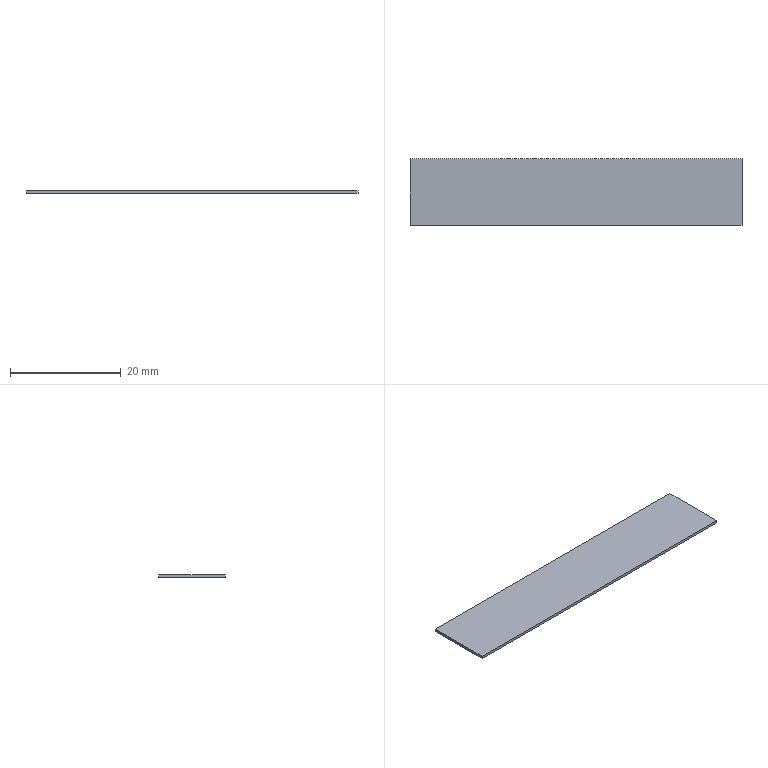Part | STEP file | 0232_013_TMEPN-2000 | 1 solid | 6 faces | box 60 x 12 x 0.5 mm | volume 359.998 mm3 | plane 6
STEP:
#1=CARTESIAN_POINT('',(0.,0.,0.));
#2=DIRECTION('',(0.,0.,1.));
#3=DIRECTION('',(1.,0.,0.));
#4=AXIS2_PLACEMENT_3D('',#1,#2,#3);
#5=CARTESIAN_POINT('',(0.,0.,0.));
#6=VERTEX_POINT('',#5);
#7=CARTESIAN_POINT('',(60.,0.,0.));
#8=VERTEX_POINT('',#7);
#9=CARTESIAN_POINT('',(60.,0.,0.));
#10=DIRECTION('',(1.,0.,0.));
#11=VECTOR('',#10,1.);
#12=LINE('',#9,#11);
#13=CARTESIAN_POINT('',(60.,6.,0.));
#14=DIRECTION('',(0.,0.,1.));
#15=DIRECTION('',(1.,0.,0.));
#16=AXIS2_PLACEMENT_3D('',#13,#14,#15);
#17=PLANE('',#16);
#18=CARTESIAN_POINT('',(0.,-6.));
#19=DIRECTION('',(1.,0.));
#20=VECTOR('',#19,1.);
#21=LINE('',#18,#20);
#22=(GEOMETRIC_REPRESENTATION_CONTEXT(2)PARAMETRIC_REPRESENTATION_CONTEXT()REPRESENTATION_CONTEXT('',''));
#23=DEFINITIONAL_REPRESENTATION('',(#21),#22);
#24=PCURVE('',#17,#23);
#25=CARTESIAN_POINT('',(1.,0.,0.));
#26=DIRECTION('',(0.,-1.,0.));
#27=DIRECTION('',(0.,0.,-1.));
#28=AXIS2_PLACEMENT_3D('',#25,#26,#27);
#29=PLANE('',#28);
#30=CARTESIAN_POINT('',(0.,59.));
#31=DIRECTION('',(0.,1.));
#32=VECTOR('',#31,1.);
#33=LINE('',#30,#32);
#34=(GEOMETRIC_REPRESENTATION_CONTEXT(2)PARAMETRIC_REPRESENTATION_CONTEXT()REPRESENTATION_CONTEXT('',''));
#35=DEFINITIONAL_REPRESENTATION('',(#33),#34);
#36=PCURVE('',#29,#35);
#37=SURFACE_CURVE('',#12,(#24,#36),.PCURVE_S1.);
#38=EDGE_CURVE('',#6,#8,#37,.T.);
#39=ORIENTED_EDGE('',*,*,#38,.F.);
#40=CARTESIAN_POINT('',(0.,12.,0.));
#41=VERTEX_POINT('',#40);
#42=CARTESIAN_POINT('',(0.,6.,0.));
#43=DIRECTION('',(0.,-1.,0.));
#44=VECTOR('',#43,1.);
#45=LINE('',#42,#44);
#46=CARTESIAN_POINT('',(-60.,0.));
#47=DIRECTION('',(0.,-1.));
#48=VECTOR('',#47,1.);
#49=LINE('',#46,#48);
#50=(GEOMETRIC_REPRESENTATION_CONTEXT(2)PARAMETRIC_REPRESENTATION_CONTEXT()REPRESENTATION_CONTEXT('',''));
#51=DEFINITIONAL_REPRESENTATION('',(#49),#50);
#52=PCURVE('',#17,#51);
#53=CARTESIAN_POINT('',(0.,0.,0.));
#54=DIRECTION('',(-1.,0.,0.));
#55=DIRECTION('',(0.,0.,1.));
#56=AXIS2_PLACEMENT_3D('',#53,#54,#55);
#57=PLANE('',#56);
#58=CARTESIAN_POINT('',(0.,6.));
#59=DIRECTION('',(0.,-1.));
#60=VECTOR('',#59,1.);
#61=LINE('',#58,#60);
#62=(GEOMETRIC_REPRESENTATION_CONTEXT(2)PARAMETRIC_REPRESENTATION_CONTEXT()REPRESENTATION_CONTEXT('',''));
#63=DEFINITIONAL_REPRESENTATION('',(#61),#62);
#64=PCURVE('',#57,#63);
#65=SURFACE_CURVE('',#45,(#52,#64),.PCURVE_S1.);
#66=EDGE_CURVE('',#41,#6,#65,.T.);
#67=ORIENTED_EDGE('',*,*,#66,.F.);
#68=CARTESIAN_POINT('',(60.,12.,0.));
#69=VERTEX_POINT('',#68);
#70=CARTESIAN_POINT('',(60.,12.,0.));
#71=DIRECTION('',(-1.,0.,0.));
#72=VECTOR('',#71,1.);
#73=LINE('',#70,#72);
#74=CARTESIAN_POINT('',(0.,6.));
#75=DIRECTION('',(-1.,0.));
#76=VECTOR('',#75,1.);
#77=LINE('',#74,#76);
#78=(GEOMETRIC_REPRESENTATION_CONTEXT(2)PARAMETRIC_REPRESENTATION_CONTEXT()REPRESENTATION_CONTEXT('',''));
#79=DEFINITIONAL_REPRESENTATION('',(#77),#78);
#80=PCURVE('',#17,#79);
#81=CARTESIAN_POINT('',(119.,12.,0.));
#82=DIRECTION('',(0.,1.,0.));
#83=DIRECTION('',(0.,0.,1.));
#84=AXIS2_PLACEMENT_3D('',#81,#82,#83);
#85=PLANE('',#84);
#86=CARTESIAN_POINT('',(0.,-59.));
#87=DIRECTION('',(0.,-1.));
#88=VECTOR('',#87,1.);
#89=LINE('',#86,#88);
#90=(GEOMETRIC_REPRESENTATION_CONTEXT(2)PARAMETRIC_REPRESENTATION_CONTEXT()REPRESENTATION_CONTEXT('',''));
#91=DEFINITIONAL_REPRESENTATION('',(#89),#90);
#92=PCURVE('',#85,#91);
#93=SURFACE_CURVE('',#73,(#80,#92),.PCURVE_S1.);
#94=EDGE_CURVE('',#69,#41,#93,.T.);
#95=ORIENTED_EDGE('',*,*,#94,.F.);
#96=CARTESIAN_POINT('',(60.,6.,0.));
#97=DIRECTION('',(0.,1.,0.));
#98=VECTOR('',#97,1.);
#99=LINE('',#96,#98);
#100=CARTESIAN_POINT('',(-0.00012,0.));
#101=DIRECTION('',(0.,1.));
#102=VECTOR('',#101,1.);
#103=LINE('',#100,#102);
#104=(GEOMETRIC_REPRESENTATION_CONTEXT(2)PARAMETRIC_REPRESENTATION_CONTEXT()REPRESENTATION_CONTEXT('',''));
#105=DEFINITIONAL_REPRESENTATION('',(#103),#104);
#106=PCURVE('',#17,#105);
#107=CARTESIAN_POINT('',(60.,12.,0.5));
#108=DIRECTION('',(-1.,0.,0.));
#109=DIRECTION('',(0.,0.,1.));
#110=AXIS2_PLACEMENT_3D('',#107,#108,#109);
#111=PLANE('',#110);
#112=CARTESIAN_POINT('',(-0.5,-6.));
#113=DIRECTION('',(0.,1.));
#114=VECTOR('',#113,1.);
#115=LINE('',#112,#114);
#116=(GEOMETRIC_REPRESENTATION_CONTEXT(2)PARAMETRIC_REPRESENTATION_CONTEXT()REPRESENTATION_CONTEXT('',''));
#117=DEFINITIONAL_REPRESENTATION('',(#115),#116);
#118=PCURVE('',#111,#117);
#119=SURFACE_CURVE('',#99,(#106,#118),.PCURVE_S1.);
#120=EDGE_CURVE('',#8,#69,#119,.T.);
#121=ORIENTED_EDGE('',*,*,#120,.F.);
#122=EDGE_LOOP('',(#39,#67,#95,#121));
#123=FACE_BOUND('',#122,.T.);
#124=ADVANCED_FACE('',(#123),#17,.F.);
#125=CARTESIAN_POINT('',(60.,12.,0.5));
#126=VERTEX_POINT('',#125);
#127=CARTESIAN_POINT('',(60.,12.,0.5));
#128=DIRECTION('',(0.,0.,-1.));
#129=VECTOR('',#128,1.);
#130=LINE('',#127,#129);
#131=CARTESIAN_POINT('',(0.,0.));
#132=DIRECTION('',(-1.,0.));
#133=VECTOR('',#132,1.);
#134=LINE('',#131,#133);
#135=(GEOMETRIC_REPRESENTATION_CONTEXT(2)PARAMETRIC_REPRESENTATION_CONTEXT()REPRESENTATION_CONTEXT('',''));
#136=DEFINITIONAL_REPRESENTATION('',(#134),#135);
#137=PCURVE('',#111,#136);
#138=CARTESIAN_POINT('',(0.5,-59.));
#139=DIRECTION('',(-1.,0.));
#140=VECTOR('',#139,1.);
#141=LINE('',#138,#140);
#142=(GEOMETRIC_REPRESENTATION_CONTEXT(2)PARAMETRIC_REPRESENTATION_CONTEXT()REPRESENTATION_CONTEXT('',''));
#143=DEFINITIONAL_REPRESENTATION('',(#141),#142);
#144=PCURVE('',#85,#143);
#145=SURFACE_CURVE('',#130,(#137,#144),.PCURVE_S1.);
#146=EDGE_CURVE('',#126,#69,#145,.T.);
#147=ORIENTED_EDGE('',*,*,#146,.F.);
#148=CARTESIAN_POINT('',(60.,0.,0.5));
#149=VERTEX_POINT('',#148);
#150=CARTESIAN_POINT('',(60.,12.,0.5));
#151=DIRECTION('',(0.,1.,0.));
#152=VECTOR('',#151,1.);
#153=LINE('',#150,#152);
#154=CARTESIAN_POINT('',(0.,0.));
#155=DIRECTION('',(0.,1.));
#156=VECTOR('',#155,1.);
#157=LINE('',#154,#156);
#158=(GEOMETRIC_REPRESENTATION_CONTEXT(2)PARAMETRIC_REPRESENTATION_CONTEXT()REPRESENTATION_CONTEXT('',''));
#159=DEFINITIONAL_REPRESENTATION('',(#157),#158);
#160=PCURVE('',#111,#159);
#161=CARTESIAN_POINT('',(60.,6.,0.5));
#162=DIRECTION('',(0.,0.,1.));
#163=DIRECTION('',(1.,0.,0.));
#164=AXIS2_PLACEMENT_3D('',#161,#162,#163);
#165=PLANE('',#164);
#166=CARTESIAN_POINT('',(-0.00012,6.));
#167=DIRECTION('',(0.,1.));
#168=VECTOR('',#167,1.);
#169=LINE('',#166,#168);
#170=(GEOMETRIC_REPRESENTATION_CONTEXT(2)PARAMETRIC_REPRESENTATION_CONTEXT()REPRESENTATION_CONTEXT('',''));
#171=DEFINITIONAL_REPRESENTATION('',(#169),#170);
#172=PCURVE('',#165,#171);
#173=SURFACE_CURVE('',#153,(#160,#172),.PCURVE_S1.);
#174=EDGE_CURVE('',#149,#126,#173,.T.);
#175=ORIENTED_EDGE('',*,*,#174,.F.);
#176=CARTESIAN_POINT('',(60.,0.,0.5));
#177=DIRECTION('',(0.,0.,1.));
#178=VECTOR('',#177,1.);
#179=LINE('',#176,#178);
#180=CARTESIAN_POINT('',(0.,-12.));
#181=DIRECTION('',(1.,0.));
#182=VECTOR('',#181,1.);
#183=LINE('',#180,#182);
#184=(GEOMETRIC_REPRESENTATION_CONTEXT(2)PARAMETRIC_REPRESENTATION_CONTEXT()REPRESENTATION_CONTEXT('',''));
#185=DEFINITIONAL_REPRESENTATION('',(#183),#184);
#186=PCURVE('',#111,#185);
#187=CARTESIAN_POINT('',(-0.5,59.));
#188=DIRECTION('',(-1.,0.));
#189=VECTOR('',#188,1.);
#190=LINE('',#187,#189);
#191=(GEOMETRIC_REPRESENTATION_CONTEXT(2)PARAMETRIC_REPRESENTATION_CONTEXT()REPRESENTATION_CONTEXT('',''));
#192=DEFINITIONAL_REPRESENTATION('',(#190),#191);
#193=PCURVE('',#29,#192);
#194=SURFACE_CURVE('',#179,(#186,#193),.PCURVE_S1.);
#195=EDGE_CURVE('',#8,#149,#194,.T.);
#196=ORIENTED_EDGE('',*,*,#195,.F.);
#197=ORIENTED_EDGE('',*,*,#120,.T.);
#198=EDGE_LOOP('',(#147,#175,#196,#197));
#199=FACE_BOUND('',#198,.T.);
#200=ADVANCED_FACE('',(#199),#111,.F.);
#201=CARTESIAN_POINT('',(0.,0.,0.5));
#202=VERTEX_POINT('',#201);
#203=CARTESIAN_POINT('',(0.,0.,0.));
#204=DIRECTION('',(0.,0.,-1.));
#205=VECTOR('',#204,1.);
#206=LINE('',#203,#205);
#207=CARTESIAN_POINT('',(0.,-1.));
#208=DIRECTION('',(1.,0.));
#209=VECTOR('',#208,1.);
#210=LINE('',#207,#209);
#211=(GEOMETRIC_REPRESENTATION_CONTEXT(2)PARAMETRIC_REPRESENTATION_CONTEXT()REPRESENTATION_CONTEXT('',''));
#212=DEFINITIONAL_REPRESENTATION('',(#210),#211);
#213=PCURVE('',#29,#212);
#214=CARTESIAN_POINT('',(0.,0.));
#215=DIRECTION('',(-1.,0.));
#216=VECTOR('',#215,1.);
#217=LINE('',#214,#216);
#218=(GEOMETRIC_REPRESENTATION_CONTEXT(2)PARAMETRIC_REPRESENTATION_CONTEXT()REPRESENTATION_CONTEXT('',''));
#219=DEFINITIONAL_REPRESENTATION('',(#217),#218);
#220=PCURVE('',#57,#219);
#221=SURFACE_CURVE('',#206,(#213,#220),.PCURVE_S1.);
#222=EDGE_CURVE('',#202,#6,#221,.T.);
#223=ORIENTED_EDGE('',*,*,#222,.T.);
#224=ORIENTED_EDGE('',*,*,#38,.T.);
#225=ORIENTED_EDGE('',*,*,#195,.T.);
#226=CARTESIAN_POINT('',(1.,0.,0.5));
#227=DIRECTION('',(-1.,0.,0.));
#228=VECTOR('',#227,1.);
#229=LINE('',#226,#228);
#230=CARTESIAN_POINT('',(-0.5,0.));
#231=DIRECTION('',(0.,-1.));
#232=VECTOR('',#231,1.);
#233=LINE('',#230,#232);
#234=(GEOMETRIC_REPRESENTATION_CONTEXT(2)PARAMETRIC_REPRESENTATION_CONTEXT()REPRESENTATION_CONTEXT('',''));
#235=DEFINITIONAL_REPRESENTATION('',(#233),#234);
#236=PCURVE('',#29,#235);
#237=CARTESIAN_POINT('',(-59.,-6.));
#238=DIRECTION('',(-1.,0.));
#239=VECTOR('',#238,1.);
#240=LINE('',#237,#239);
#241=(GEOMETRIC_REPRESENTATION_CONTEXT(2)PARAMETRIC_REPRESENTATION_CONTEXT()REPRESENTATION_CONTEXT('',''));
#242=DEFINITIONAL_REPRESENTATION('',(#240),#241);
#243=PCURVE('',#165,#242);
#244=SURFACE_CURVE('',#229,(#236,#243),.PCURVE_S1.);
#245=EDGE_CURVE('',#149,#202,#244,.T.);
#246=ORIENTED_EDGE('',*,*,#245,.T.);
#247=EDGE_LOOP('',(#223,#224,#225,#246));
#248=FACE_BOUND('',#247,.T.);
#249=ADVANCED_FACE('',(#248),#29,.T.);
#250=ORIENTED_EDGE('',*,*,#66,.T.);
#251=ORIENTED_EDGE('',*,*,#222,.F.);
#252=CARTESIAN_POINT('',(0.,12.,0.5));
#253=VERTEX_POINT('',#252);
#254=CARTESIAN_POINT('',(0.,0.,0.5));
#255=DIRECTION('',(0.,1.,0.));
#256=VECTOR('',#255,1.);
#257=LINE('',#254,#256);
#258=CARTESIAN_POINT('',(0.5,0.));
#259=DIRECTION('',(0.,1.));
#260=VECTOR('',#259,1.);
#261=LINE('',#258,#260);
#262=(GEOMETRIC_REPRESENTATION_CONTEXT(2)PARAMETRIC_REPRESENTATION_CONTEXT()REPRESENTATION_CONTEXT('',''));
#263=DEFINITIONAL_REPRESENTATION('',(#261),#262);
#264=PCURVE('',#57,#263);
#265=CARTESIAN_POINT('',(-60.,-6.));
#266=DIRECTION('',(0.,1.));
#267=VECTOR('',#266,1.);
#268=LINE('',#265,#267);
#269=(GEOMETRIC_REPRESENTATION_CONTEXT(2)PARAMETRIC_REPRESENTATION_CONTEXT()REPRESENTATION_CONTEXT('',''));
#270=DEFINITIONAL_REPRESENTATION('',(#268),#269);
#271=PCURVE('',#165,#270);
#272=SURFACE_CURVE('',#257,(#264,#271),.PCURVE_S1.);
#273=EDGE_CURVE('',#202,#253,#272,.T.);
#274=ORIENTED_EDGE('',*,*,#273,.T.);
#275=CARTESIAN_POINT('',(0.,12.,0.));
#276=DIRECTION('',(0.,0.,-1.));
#277=VECTOR('',#276,1.);
#278=LINE('',#275,#277);
#279=CARTESIAN_POINT('',(0.,12.));
#280=DIRECTION('',(-1.,0.));
#281=VECTOR('',#280,1.);
#282=LINE('',#279,#281);
#283=(GEOMETRIC_REPRESENTATION_CONTEXT(2)PARAMETRIC_REPRESENTATION_CONTEXT()REPRESENTATION_CONTEXT('',''));
#284=DEFINITIONAL_REPRESENTATION('',(#282),#283);
#285=PCURVE('',#57,#284);
#286=CARTESIAN_POINT('',(0.,-119.));
#287=DIRECTION('',(-1.,0.));
#288=VECTOR('',#287,1.);
#289=LINE('',#286,#288);
#290=(GEOMETRIC_REPRESENTATION_CONTEXT(2)PARAMETRIC_REPRESENTATION_CONTEXT()REPRESENTATION_CONTEXT('',''));
#291=DEFINITIONAL_REPRESENTATION('',(#289),#290);
#292=PCURVE('',#85,#291);
#293=SURFACE_CURVE('',#278,(#285,#292),.PCURVE_S1.);
#294=EDGE_CURVE('',#253,#41,#293,.T.);
#295=ORIENTED_EDGE('',*,*,#294,.T.);
#296=EDGE_LOOP('',(#250,#251,#274,#295));
#297=FACE_BOUND('',#296,.T.);
#298=ADVANCED_FACE('',(#297),#57,.T.);
#299=ORIENTED_EDGE('',*,*,#294,.F.);
#300=CARTESIAN_POINT('',(119.,12.,0.5));
#301=DIRECTION('',(1.,0.,0.));
#302=VECTOR('',#301,1.);
#303=LINE('',#300,#302);
#304=CARTESIAN_POINT('',(0.5,0.));
#305=DIRECTION('',(0.,1.));
#306=VECTOR('',#305,1.);
#307=LINE('',#304,#306);
#308=(GEOMETRIC_REPRESENTATION_CONTEXT(2)PARAMETRIC_REPRESENTATION_CONTEXT()REPRESENTATION_CONTEXT('',''));
#309=DEFINITIONAL_REPRESENTATION('',(#307),#308);
#310=PCURVE('',#85,#309);
#311=CARTESIAN_POINT('',(59.,6.));
#312=DIRECTION('',(1.,0.));
#313=VECTOR('',#312,1.);
#314=LINE('',#311,#313);
#315=(GEOMETRIC_REPRESENTATION_CONTEXT(2)PARAMETRIC_REPRESENTATION_CONTEXT()REPRESENTATION_CONTEXT('',''));
#316=DEFINITIONAL_REPRESENTATION('',(#314),#315);
#317=PCURVE('',#165,#316);
#318=SURFACE_CURVE('',#303,(#310,#317),.PCURVE_S1.);
#319=EDGE_CURVE('',#253,#126,#318,.T.);
#320=ORIENTED_EDGE('',*,*,#319,.T.);
#321=ORIENTED_EDGE('',*,*,#146,.T.);
#322=ORIENTED_EDGE('',*,*,#94,.T.);
#323=EDGE_LOOP('',(#299,#320,#321,#322));
#324=FACE_BOUND('',#323,.T.);
#325=ADVANCED_FACE('',(#324),#85,.T.);
#326=ORIENTED_EDGE('',*,*,#273,.F.);
#327=ORIENTED_EDGE('',*,*,#245,.F.);
#328=ORIENTED_EDGE('',*,*,#174,.T.);
#329=ORIENTED_EDGE('',*,*,#319,.F.);
#330=EDGE_LOOP('',(#326,#327,#328,#329));
#331=FACE_BOUND('',#330,.T.);
#332=ADVANCED_FACE('',(#331),#165,.T.);
#333=CLOSED_SHELL('',(#124,#200,#249,#298,#325,#332));
#334=MANIFOLD_SOLID_BREP('',#333);
#335=(LENGTH_UNIT()NAMED_UNIT(*)SI_UNIT(.MILLI.,.METRE.));
#336=UNCERTAINTY_MEASURE_WITH_UNIT(LENGTH_MEASURE(0.0000001),#335,'','');
#337=(NAMED_UNIT(*)PLANE_ANGLE_UNIT()SI_UNIT($,.RADIAN.));
#338=(NAMED_UNIT(*)SI_UNIT($,.STERADIAN.)SOLID_ANGLE_UNIT());
#339=(GEOMETRIC_REPRESENTATION_CONTEXT(3)GLOBAL_UNCERTAINTY_ASSIGNED_CONTEXT((#336))GLOBAL_UNIT_ASSIGNED_CONTEXT((#335,#337,#338))REPRESENTATION_CONTEXT('',''));
#340=ADVANCED_BREP_SHAPE_REPRESENTATION('',(#4,#334),#339);